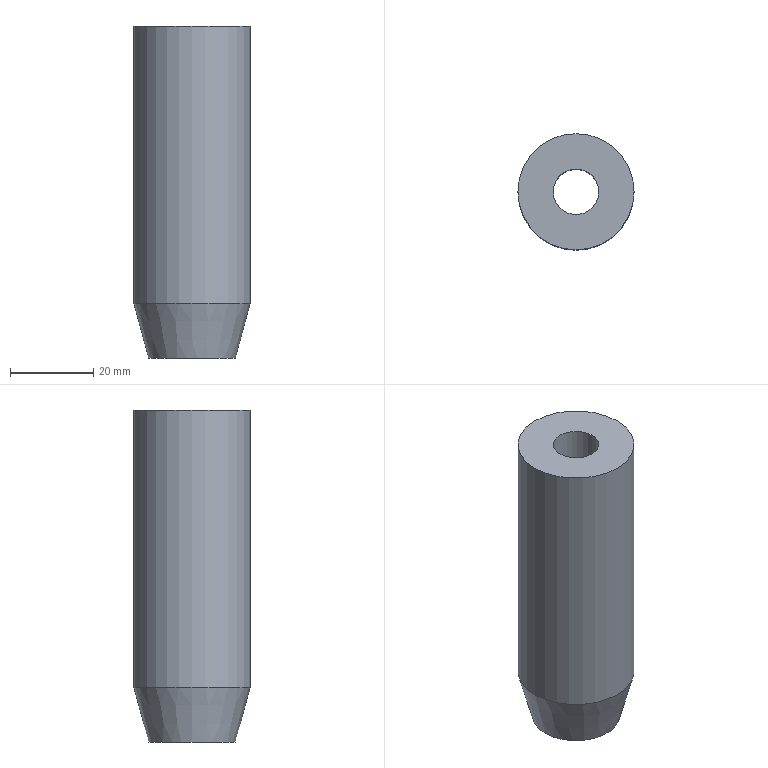Part | NX | features solid 2 | 1 solid | 5 faces | box 28 x 28 x 80 mm | volume 39777 mm3 | plane 2 | cylinder 2 | cone 1 | commonest cylinder face diameters 11 x1 28 x1
STEP:
#1=CARTESIAN_POINT('',(-321.,270.,220.));
#2=VERTEX_POINT('',#1);
#3=CARTESIAN_POINT('',(-335.,270.,220.));
#4=DIRECTION('',(0.,0.,1.));
#5=DIRECTION('',(1.,0.,0.));
#6=AXIS2_PLACEMENT_3D('',#3,#4,#5);
#7=CIRCLE('',#6,14.);
#8=EDGE_CURVE('',#2,#2,#7,.T.);
#9=ORIENTED_EDGE('',*,*,#8,.T.);
#10=EDGE_LOOP('',(#9));
#11=FACE_BOUND('',#10,.T.);
#12=CARTESIAN_POINT('',(-329.5,270.,220.));
#13=VERTEX_POINT('',#12);
#14=CARTESIAN_POINT('',(-335.,270.,220.));
#15=DIRECTION('',(0.,0.,1.));
#16=DIRECTION('',(1.,0.,0.));
#17=AXIS2_PLACEMENT_3D('',#14,#15,#16);
#18=CIRCLE('',#17,5.5);
#19=EDGE_CURVE('',#13,#13,#18,.T.);
#20=ORIENTED_EDGE('',*,*,#19,.F.);
#21=EDGE_LOOP('',(#20));
#22=FACE_BOUND('',#21,.T.);
#23=CARTESIAN_POINT('',(-335.,270.,220.));
#24=DIRECTION('',(0.,0.,1.));
#25=DIRECTION('',(1.,0.,0.));
#26=AXIS2_PLACEMENT_3D('',#23,#24,#25);
#27=PLANE('',#26);
#28=ADVANCED_FACE('',(#11,#22),#27,.T.);
#29=CARTESIAN_POINT('',(-324.537,270.,140.));
#30=VERTEX_POINT('',#29);
#31=CARTESIAN_POINT('',(-335.,270.,140.));
#32=DIRECTION('',(0.,0.,1.));
#33=DIRECTION('',(1.,0.,0.));
#34=AXIS2_PLACEMENT_3D('',#31,#32,#33);
#35=CIRCLE('',#34,10.463);
#36=EDGE_CURVE('',#30,#30,#35,.F.);
#37=ORIENTED_EDGE('',*,*,#36,.T.);
#38=EDGE_LOOP('',(#37));
#39=FACE_BOUND('',#38,.T.);
#40=CARTESIAN_POINT('',(-329.5,270.,140.));
#41=VERTEX_POINT('',#40);
#42=CARTESIAN_POINT('',(-335.,270.,140.));
#43=DIRECTION('',(0.,0.,1.));
#44=DIRECTION('',(1.,0.,0.));
#45=AXIS2_PLACEMENT_3D('',#42,#43,#44);
#46=CIRCLE('',#45,5.5);
#47=EDGE_CURVE('',#41,#41,#46,.T.);
#48=ORIENTED_EDGE('',*,*,#47,.T.);
#49=EDGE_LOOP('',(#48));
#50=FACE_BOUND('',#49,.T.);
#51=CARTESIAN_POINT('',(-335.,270.,140.));
#52=DIRECTION('',(0.,0.,1.));
#53=DIRECTION('',(1.,0.,0.));
#54=AXIS2_PLACEMENT_3D('',#51,#52,#53);
#55=PLANE('',#54);
#56=ADVANCED_FACE('',(#39,#50),#55,.F.);
#57=CARTESIAN_POINT('',(-321.,270.,153.201));
#58=VERTEX_POINT('',#57);
#59=CARTESIAN_POINT('',(-335.,270.,153.201));
#60=DIRECTION('',(0.,0.,1.));
#61=DIRECTION('',(1.,0.,0.));
#62=AXIS2_PLACEMENT_3D('',#59,#60,#61);
#63=CIRCLE('',#62,14.);
#64=EDGE_CURVE('',#58,#58,#63,.T.);
#65=ORIENTED_EDGE('',*,*,#64,.T.);
#66=EDGE_LOOP('',(#65));
#67=FACE_BOUND('',#66,.T.);
#68=ORIENTED_EDGE('',*,*,#8,.F.);
#69=EDGE_LOOP('',(#68));
#70=FACE_BOUND('',#69,.T.);
#71=CARTESIAN_POINT('',(-335.,270.,200.));
#72=DIRECTION('',(0.,0.,-1.));
#73=DIRECTION('',(-1.,0.,0.));
#74=AXIS2_PLACEMENT_3D('',#71,#72,#73);
#75=CYLINDRICAL_SURFACE('',#74,14.);
#76=ADVANCED_FACE('',(#67,#70),#75,.T.);
#77=ORIENTED_EDGE('',*,*,#19,.T.);
#78=EDGE_LOOP('',(#77));
#79=FACE_BOUND('',#78,.T.);
#80=ORIENTED_EDGE('',*,*,#47,.F.);
#81=EDGE_LOOP('',(#80));
#82=FACE_BOUND('',#81,.T.);
#83=CARTESIAN_POINT('',(-335.,270.,200.));
#84=DIRECTION('',(0.,0.,-1.));
#85=DIRECTION('',(-1.,0.,0.));
#86=AXIS2_PLACEMENT_3D('',#83,#84,#85);
#87=CYLINDRICAL_SURFACE('',#86,5.5);
#88=ADVANCED_FACE('',(#79,#82),#87,.F.);
#89=ORIENTED_EDGE('',*,*,#36,.F.);
#90=EDGE_LOOP('',(#89));
#91=FACE_BOUND('',#90,.T.);
#92=ORIENTED_EDGE('',*,*,#64,.F.);
#93=EDGE_LOOP('',(#92));
#94=FACE_BOUND('',#93,.T.);
#95=CARTESIAN_POINT('',(-335.,270.,145.482));
#96=DIRECTION('',(0.,0.,1.));
#97=DIRECTION('',(1.,0.,0.));
#98=AXIS2_PLACEMENT_3D('',#95,#96,#97);
#99=CONICAL_SURFACE('',#98,11.932,0.2618);
#100=ADVANCED_FACE('',(#91,#94),#99,.T.);
#101=CLOSED_SHELL('',(#28,#56,#76,#88,#100));
#102=MANIFOLD_SOLID_BREP('',#101);
#103=(LENGTH_UNIT()NAMED_UNIT(*)SI_UNIT(.MILLI.,.METRE.));
#104=UNCERTAINTY_MEASURE_WITH_UNIT(LENGTH_MEASURE(0.00001),#103,'','');
#105=(NAMED_UNIT(*)PLANE_ANGLE_UNIT()SI_UNIT($,.RADIAN.));
#106=(NAMED_UNIT(*)SI_UNIT($,.STERADIAN.)SOLID_ANGLE_UNIT());
#107=(GEOMETRIC_REPRESENTATION_CONTEXT(3)GLOBAL_UNCERTAINTY_ASSIGNED_CONTEXT((#104))GLOBAL_UNIT_ASSIGNED_CONTEXT((#103,#105,#106))REPRESENTATION_CONTEXT('',''));
#108=ADVANCED_BREP_SHAPE_REPRESENTATION('',(#102),#107);